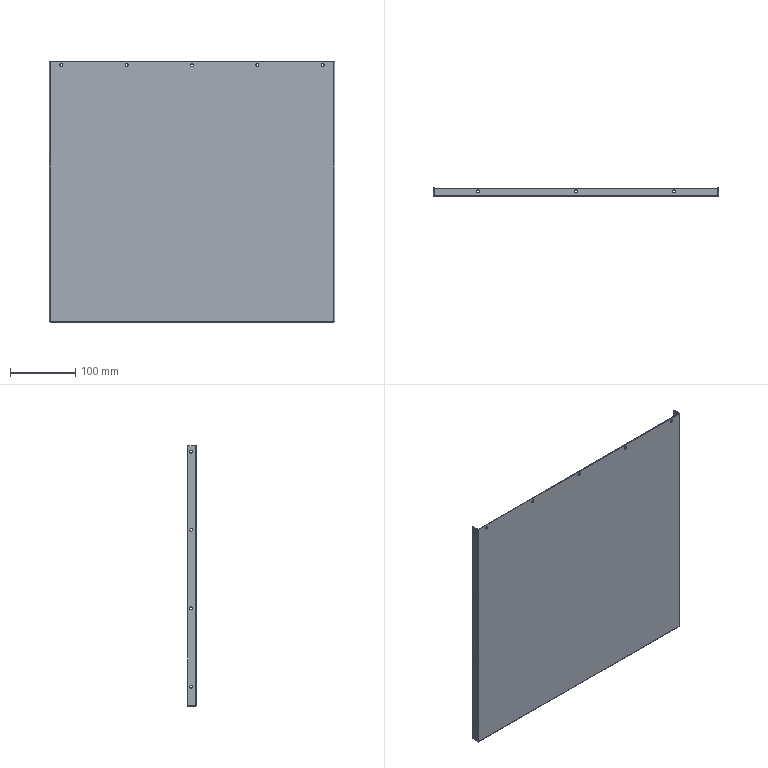Part | SolidWorks | features ICE 3, LPattern 3, EdgeFlange 1, FlatPattern 1, SMBaseFlange 1, SheetMetal 1 | 1 solid | 62 faces | box 437.001 x 12.7 x 399 mm | volume 225419 mm3 | cylinder 38 | plane 20 | spline 4 | commonest cylinder face diameters 4.5 x32 0.2 x3 2.6 x3